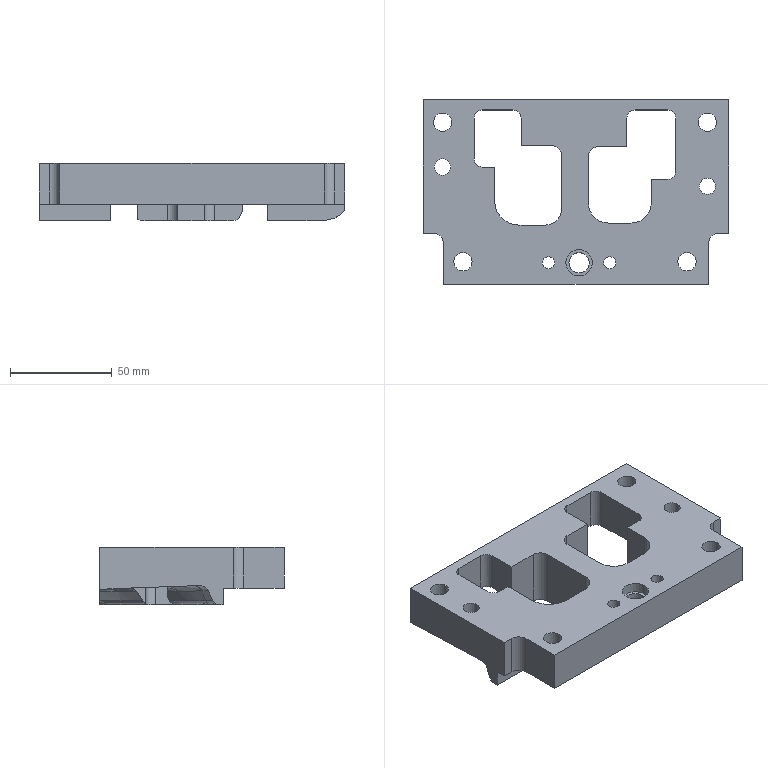Part | STEP file | 418_id1210_x_t | 1 solid | 92 faces | box 150 x 90.5 x 28 mm | volume 195768 mm3 | plane 39 | cylinder 30 | spline 23 | commonest cylinder face diameters 8 x8 9 x6 10 x5 14 x4 6 x2 20 x2